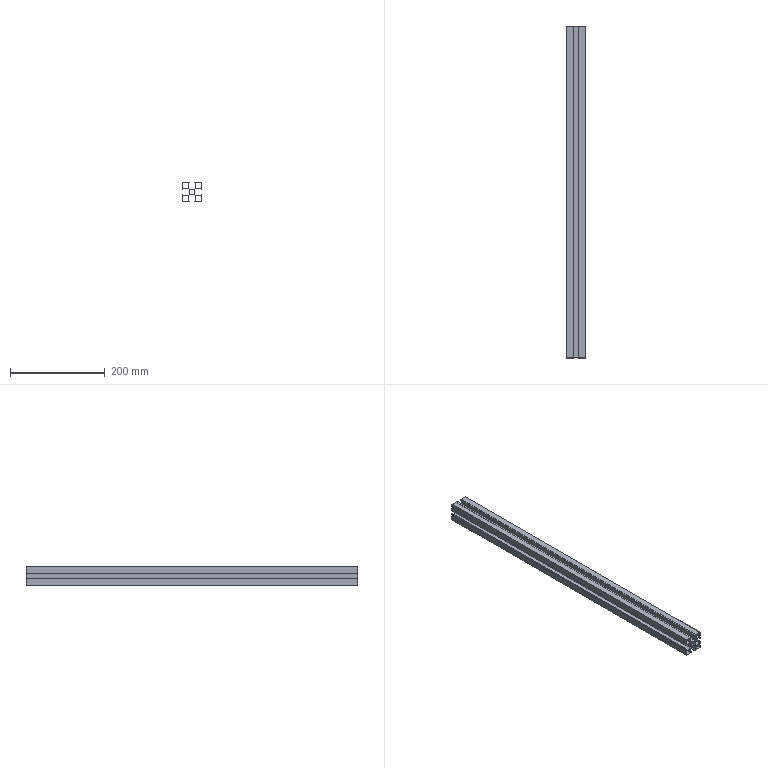Part | SolidWorks | features MirrorPattern 2, Extrusion 1 | 1 solid | 85 faces | box 40 x 700 x 40 mm | volume 182553 mm3 | plane 70 | cylinder 15 | commonest cylinder face diameters 2 x6 10.6 x5 1 x4